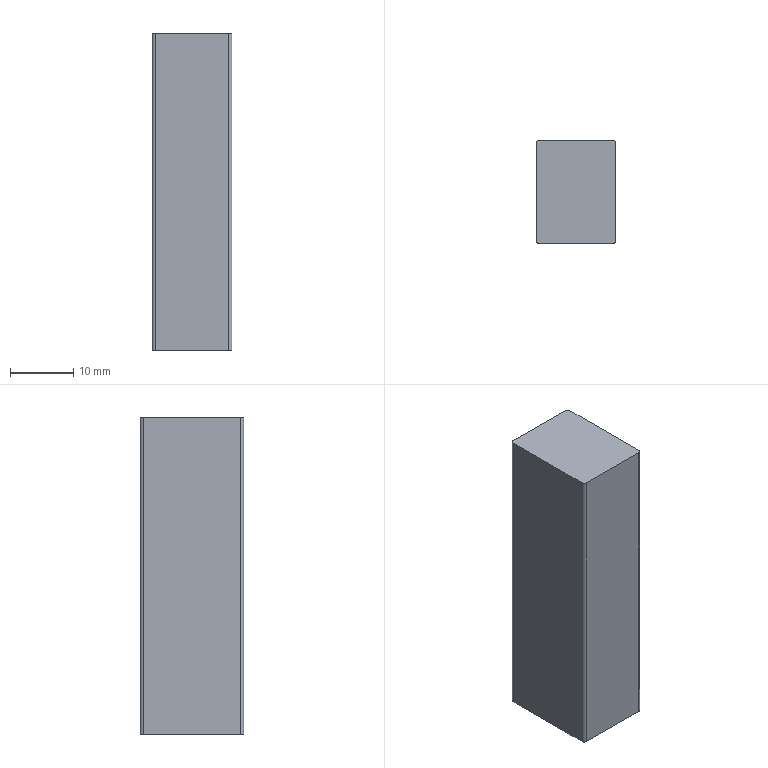Part | NX | features BREP 1 | 1 solid | 10 faces | box 12.615 x 16.326 x 50 mm | volume 10287 mm3 | plane 6 | cylinder 4 | commonest cylinder face diameters 1 x4
STEP:
#1=CARTESIAN_POINT('',(-5.808,8.163,-40.6));
#2=VERTEX_POINT('',#1);
#3=CARTESIAN_POINT('',(-6.308,7.663,-40.6));
#4=VERTEX_POINT('',#3);
#5=CARTESIAN_POINT('',(-5.808,7.663,-40.6));
#6=DIRECTION('',(0.,0.,1.));
#7=DIRECTION('',(1.,0.,0.));
#8=AXIS2_PLACEMENT_3D('',#5,#6,#7);
#9=CIRCLE('',#8,0.5);
#10=EDGE_CURVE('',#2,#4,#9,.T.);
#11=ORIENTED_EDGE('',*,*,#10,.F.);
#12=CARTESIAN_POINT('',(-5.808,8.163,-90.6));
#13=VERTEX_POINT('',#12);
#14=CARTESIAN_POINT('',(-5.808,8.163,-90.6));
#15=DIRECTION('',(0.,0.,1.));
#16=VECTOR('',#15,1000.);
#17=LINE('',#14,#16);
#18=EDGE_CURVE('',#13,#2,#17,.T.);
#19=ORIENTED_EDGE('',*,*,#18,.F.);
#20=CARTESIAN_POINT('',(-6.308,7.663,-90.6));
#21=VERTEX_POINT('',#20);
#22=CARTESIAN_POINT('',(-5.808,7.663,-90.6));
#23=DIRECTION('',(0.,0.,1.));
#24=DIRECTION('',(1.,0.,0.));
#25=AXIS2_PLACEMENT_3D('',#22,#23,#24);
#26=CIRCLE('',#25,0.5);
#27=EDGE_CURVE('',#13,#21,#26,.T.);
#28=ORIENTED_EDGE('',*,*,#27,.T.);
#29=CARTESIAN_POINT('',(-6.308,7.663,-90.6));
#30=DIRECTION('',(0.,0.,1.));
#31=VECTOR('',#30,1000.);
#32=LINE('',#29,#31);
#33=EDGE_CURVE('',#21,#4,#32,.T.);
#34=ORIENTED_EDGE('',*,*,#33,.T.);
#35=EDGE_LOOP('',(#11,#19,#28,#34));
#36=FACE_BOUND('',#35,.T.);
#37=CARTESIAN_POINT('',(-5.808,7.663,-90.6));
#38=DIRECTION('',(0.,0.,1.));
#39=DIRECTION('',(-1.,0.,0.));
#40=AXIS2_PLACEMENT_3D('',#37,#38,#39);
#41=CYLINDRICAL_SURFACE('',#40,0.5);
#42=ADVANCED_FACE('',(#36),#41,.T.);
#43=CARTESIAN_POINT('',(-6.308,-7.663,-40.6));
#44=VERTEX_POINT('',#43);
#45=CARTESIAN_POINT('',(-6.308,-7.663,-40.6));
#46=DIRECTION('',(0.,1.,0.));
#47=VECTOR('',#46,1000.);
#48=LINE('',#45,#47);
#49=EDGE_CURVE('',#44,#4,#48,.T.);
#50=ORIENTED_EDGE('',*,*,#49,.T.);
#51=ORIENTED_EDGE('',*,*,#33,.F.);
#52=CARTESIAN_POINT('',(-6.308,-7.663,-90.6));
#53=VERTEX_POINT('',#52);
#54=CARTESIAN_POINT('',(-6.308,-7.663,-90.6));
#55=DIRECTION('',(0.,1.,0.));
#56=VECTOR('',#55,1000.);
#57=LINE('',#54,#56);
#58=EDGE_CURVE('',#53,#21,#57,.T.);
#59=ORIENTED_EDGE('',*,*,#58,.F.);
#60=CARTESIAN_POINT('',(-6.308,-7.663,-90.6));
#61=DIRECTION('',(0.,0.,1.));
#62=VECTOR('',#61,1000.);
#63=LINE('',#60,#62);
#64=EDGE_CURVE('',#53,#44,#63,.T.);
#65=ORIENTED_EDGE('',*,*,#64,.T.);
#66=EDGE_LOOP('',(#50,#51,#59,#65));
#67=FACE_BOUND('',#66,.T.);
#68=CARTESIAN_POINT('',(-6.308,-7.663,-90.6));
#69=DIRECTION('',(1.,0.,0.));
#70=DIRECTION('',(0.,0.,1.));
#71=AXIS2_PLACEMENT_3D('',#68,#69,#70);
#72=PLANE('',#71);
#73=ADVANCED_FACE('',(#67),#72,.F.);
#74=CARTESIAN_POINT('',(-5.808,-8.163,-40.6));
#75=VERTEX_POINT('',#74);
#76=CARTESIAN_POINT('',(-5.808,-7.663,-40.6));
#77=DIRECTION('',(0.,0.,1.));
#78=DIRECTION('',(1.,0.,0.));
#79=AXIS2_PLACEMENT_3D('',#76,#77,#78);
#80=CIRCLE('',#79,0.5);
#81=EDGE_CURVE('',#44,#75,#80,.T.);
#82=ORIENTED_EDGE('',*,*,#81,.F.);
#83=ORIENTED_EDGE('',*,*,#64,.F.);
#84=CARTESIAN_POINT('',(-5.808,-8.163,-90.6));
#85=VERTEX_POINT('',#84);
#86=CARTESIAN_POINT('',(-5.808,-7.663,-90.6));
#87=DIRECTION('',(0.,0.,1.));
#88=DIRECTION('',(1.,0.,0.));
#89=AXIS2_PLACEMENT_3D('',#86,#87,#88);
#90=CIRCLE('',#89,0.5);
#91=EDGE_CURVE('',#53,#85,#90,.T.);
#92=ORIENTED_EDGE('',*,*,#91,.T.);
#93=CARTESIAN_POINT('',(-5.808,-8.163,-90.6));
#94=DIRECTION('',(0.,0.,1.));
#95=VECTOR('',#94,1000.);
#96=LINE('',#93,#95);
#97=EDGE_CURVE('',#85,#75,#96,.T.);
#98=ORIENTED_EDGE('',*,*,#97,.T.);
#99=EDGE_LOOP('',(#82,#83,#92,#98));
#100=FACE_BOUND('',#99,.T.);
#101=CARTESIAN_POINT('',(-5.808,-7.663,-90.6));
#102=DIRECTION('',(0.,0.,1.));
#103=DIRECTION('',(-1.,0.,0.));
#104=AXIS2_PLACEMENT_3D('',#101,#102,#103);
#105=CYLINDRICAL_SURFACE('',#104,0.5);
#106=ADVANCED_FACE('',(#100),#105,.T.);
#107=CARTESIAN_POINT('',(5.808,-8.163,-40.6));
#108=VERTEX_POINT('',#107);
#109=CARTESIAN_POINT('',(5.808,-8.163,-40.6));
#110=DIRECTION('',(-1.,0.,0.));
#111=VECTOR('',#110,1000.);
#112=LINE('',#109,#111);
#113=EDGE_CURVE('',#108,#75,#112,.T.);
#114=ORIENTED_EDGE('',*,*,#113,.T.);
#115=ORIENTED_EDGE('',*,*,#97,.F.);
#116=CARTESIAN_POINT('',(5.808,-8.163,-90.6));
#117=VERTEX_POINT('',#116);
#118=CARTESIAN_POINT('',(5.808,-8.163,-90.6));
#119=DIRECTION('',(-1.,0.,0.));
#120=VECTOR('',#119,1000.);
#121=LINE('',#118,#120);
#122=EDGE_CURVE('',#117,#85,#121,.T.);
#123=ORIENTED_EDGE('',*,*,#122,.F.);
#124=CARTESIAN_POINT('',(5.808,-8.163,-90.6));
#125=DIRECTION('',(0.,0.,1.));
#126=VECTOR('',#125,1000.);
#127=LINE('',#124,#126);
#128=EDGE_CURVE('',#117,#108,#127,.T.);
#129=ORIENTED_EDGE('',*,*,#128,.T.);
#130=EDGE_LOOP('',(#114,#115,#123,#129));
#131=FACE_BOUND('',#130,.T.);
#132=CARTESIAN_POINT('',(5.808,-8.163,-90.6));
#133=DIRECTION('',(0.,1.,0.));
#134=DIRECTION('',(0.,0.,-1.));
#135=AXIS2_PLACEMENT_3D('',#132,#133,#134);
#136=PLANE('',#135);
#137=ADVANCED_FACE('',(#131),#136,.F.);
#138=CARTESIAN_POINT('',(6.308,-7.663,-40.6));
#139=VERTEX_POINT('',#138);
#140=CARTESIAN_POINT('',(5.808,-7.663,-40.6));
#141=DIRECTION('',(0.,0.,1.));
#142=DIRECTION('',(1.,0.,0.));
#143=AXIS2_PLACEMENT_3D('',#140,#141,#142);
#144=CIRCLE('',#143,0.5);
#145=EDGE_CURVE('',#108,#139,#144,.T.);
#146=ORIENTED_EDGE('',*,*,#145,.F.);
#147=ORIENTED_EDGE('',*,*,#128,.F.);
#148=CARTESIAN_POINT('',(6.308,-7.663,-90.6));
#149=VERTEX_POINT('',#148);
#150=CARTESIAN_POINT('',(5.808,-7.663,-90.6));
#151=DIRECTION('',(0.,0.,1.));
#152=DIRECTION('',(1.,0.,0.));
#153=AXIS2_PLACEMENT_3D('',#150,#151,#152);
#154=CIRCLE('',#153,0.5);
#155=EDGE_CURVE('',#117,#149,#154,.T.);
#156=ORIENTED_EDGE('',*,*,#155,.T.);
#157=CARTESIAN_POINT('',(6.308,-7.663,-90.6));
#158=DIRECTION('',(0.,0.,1.));
#159=VECTOR('',#158,1000.);
#160=LINE('',#157,#159);
#161=EDGE_CURVE('',#149,#139,#160,.T.);
#162=ORIENTED_EDGE('',*,*,#161,.T.);
#163=EDGE_LOOP('',(#146,#147,#156,#162));
#164=FACE_BOUND('',#163,.T.);
#165=CARTESIAN_POINT('',(5.808,-7.663,-90.6));
#166=DIRECTION('',(0.,0.,1.));
#167=DIRECTION('',(-1.,0.,0.));
#168=AXIS2_PLACEMENT_3D('',#165,#166,#167);
#169=CYLINDRICAL_SURFACE('',#168,0.5);
#170=ADVANCED_FACE('',(#164),#169,.T.);
#171=CARTESIAN_POINT('',(6.308,7.663,-40.6));
#172=VERTEX_POINT('',#171);
#173=CARTESIAN_POINT('',(6.308,7.663,-40.6));
#174=DIRECTION('',(0.,-1.,0.));
#175=VECTOR('',#174,1000.);
#176=LINE('',#173,#175);
#177=EDGE_CURVE('',#172,#139,#176,.T.);
#178=ORIENTED_EDGE('',*,*,#177,.T.);
#179=ORIENTED_EDGE('',*,*,#161,.F.);
#180=CARTESIAN_POINT('',(6.308,7.663,-90.6));
#181=VERTEX_POINT('',#180);
#182=CARTESIAN_POINT('',(6.308,7.663,-90.6));
#183=DIRECTION('',(0.,-1.,0.));
#184=VECTOR('',#183,1000.);
#185=LINE('',#182,#184);
#186=EDGE_CURVE('',#181,#149,#185,.T.);
#187=ORIENTED_EDGE('',*,*,#186,.F.);
#188=CARTESIAN_POINT('',(6.308,7.663,-90.6));
#189=DIRECTION('',(0.,0.,1.));
#190=VECTOR('',#189,1000.);
#191=LINE('',#188,#190);
#192=EDGE_CURVE('',#181,#172,#191,.T.);
#193=ORIENTED_EDGE('',*,*,#192,.T.);
#194=EDGE_LOOP('',(#178,#179,#187,#193));
#195=FACE_BOUND('',#194,.T.);
#196=CARTESIAN_POINT('',(6.308,7.663,-90.6));
#197=DIRECTION('',(-1.,0.,0.));
#198=DIRECTION('',(0.,1.,0.));
#199=AXIS2_PLACEMENT_3D('',#196,#197,#198);
#200=PLANE('',#199);
#201=ADVANCED_FACE('',(#195),#200,.F.);
#202=CARTESIAN_POINT('',(5.808,8.163,-40.6));
#203=VERTEX_POINT('',#202);
#204=CARTESIAN_POINT('',(5.808,7.663,-40.6));
#205=DIRECTION('',(0.,0.,1.));
#206=DIRECTION('',(1.,0.,0.));
#207=AXIS2_PLACEMENT_3D('',#204,#205,#206);
#208=CIRCLE('',#207,0.5);
#209=EDGE_CURVE('',#172,#203,#208,.T.);
#210=ORIENTED_EDGE('',*,*,#209,.F.);
#211=ORIENTED_EDGE('',*,*,#192,.F.);
#212=CARTESIAN_POINT('',(5.808,8.163,-90.6));
#213=VERTEX_POINT('',#212);
#214=CARTESIAN_POINT('',(5.808,7.663,-90.6));
#215=DIRECTION('',(0.,0.,1.));
#216=DIRECTION('',(1.,0.,0.));
#217=AXIS2_PLACEMENT_3D('',#214,#215,#216);
#218=CIRCLE('',#217,0.5);
#219=EDGE_CURVE('',#181,#213,#218,.T.);
#220=ORIENTED_EDGE('',*,*,#219,.T.);
#221=CARTESIAN_POINT('',(5.808,8.163,-90.6));
#222=DIRECTION('',(0.,0.,1.));
#223=VECTOR('',#222,1000.);
#224=LINE('',#221,#223);
#225=EDGE_CURVE('',#213,#203,#224,.T.);
#226=ORIENTED_EDGE('',*,*,#225,.T.);
#227=EDGE_LOOP('',(#210,#211,#220,#226));
#228=FACE_BOUND('',#227,.T.);
#229=CARTESIAN_POINT('',(5.808,7.663,-90.6));
#230=DIRECTION('',(0.,0.,1.));
#231=DIRECTION('',(-1.,0.,0.));
#232=AXIS2_PLACEMENT_3D('',#229,#230,#231);
#233=CYLINDRICAL_SURFACE('',#232,0.5);
#234=ADVANCED_FACE('',(#228),#233,.T.);
#235=CARTESIAN_POINT('',(-5.808,8.163,-40.6));
#236=DIRECTION('',(1.,0.,0.));
#237=VECTOR('',#236,1000.);
#238=LINE('',#235,#237);
#239=EDGE_CURVE('',#2,#203,#238,.T.);
#240=ORIENTED_EDGE('',*,*,#239,.T.);
#241=ORIENTED_EDGE('',*,*,#225,.F.);
#242=CARTESIAN_POINT('',(-5.808,8.163,-90.6));
#243=DIRECTION('',(1.,0.,0.));
#244=VECTOR('',#243,1000.);
#245=LINE('',#242,#244);
#246=EDGE_CURVE('',#13,#213,#245,.T.);
#247=ORIENTED_EDGE('',*,*,#246,.F.);
#248=ORIENTED_EDGE('',*,*,#18,.T.);
#249=EDGE_LOOP('',(#240,#241,#247,#248));
#250=FACE_BOUND('',#249,.T.);
#251=CARTESIAN_POINT('',(-5.808,8.163,-90.6));
#252=DIRECTION('',(0.,-1.,0.));
#253=DIRECTION('',(-1.,0.,0.));
#254=AXIS2_PLACEMENT_3D('',#251,#252,#253);
#255=PLANE('',#254);
#256=ADVANCED_FACE('',(#250),#255,.F.);
#257=ORIENTED_EDGE('',*,*,#27,.F.);
#258=ORIENTED_EDGE('',*,*,#246,.T.);
#259=ORIENTED_EDGE('',*,*,#219,.F.);
#260=ORIENTED_EDGE('',*,*,#186,.T.);
#261=ORIENTED_EDGE('',*,*,#155,.F.);
#262=ORIENTED_EDGE('',*,*,#122,.T.);
#263=ORIENTED_EDGE('',*,*,#91,.F.);
#264=ORIENTED_EDGE('',*,*,#58,.T.);
#265=EDGE_LOOP('',(#257,#258,#259,#260,#261,#262,#263,#264));
#266=FACE_BOUND('',#265,.T.);
#267=CARTESIAN_POINT('',(-5.808,7.663,-90.6));
#268=DIRECTION('',(0.,0.,1.));
#269=DIRECTION('',(-1.,0.,0.));
#270=AXIS2_PLACEMENT_3D('',#267,#268,#269);
#271=PLANE('',#270);
#272=ADVANCED_FACE('',(#266),#271,.F.);
#273=ORIENTED_EDGE('',*,*,#10,.T.);
#274=ORIENTED_EDGE('',*,*,#49,.F.);
#275=ORIENTED_EDGE('',*,*,#81,.T.);
#276=ORIENTED_EDGE('',*,*,#113,.F.);
#277=ORIENTED_EDGE('',*,*,#145,.T.);
#278=ORIENTED_EDGE('',*,*,#177,.F.);
#279=ORIENTED_EDGE('',*,*,#209,.T.);
#280=ORIENTED_EDGE('',*,*,#239,.F.);
#281=EDGE_LOOP('',(#273,#274,#275,#276,#277,#278,#279,#280));
#282=FACE_BOUND('',#281,.T.);
#283=CARTESIAN_POINT('',(-5.808,7.663,-40.6));
#284=DIRECTION('',(0.,0.,1.));
#285=DIRECTION('',(-1.,0.,0.));
#286=AXIS2_PLACEMENT_3D('',#283,#284,#285);
#287=PLANE('',#286);
#288=ADVANCED_FACE('',(#282),#287,.T.);
#289=CLOSED_SHELL('',(#42,#73,#106,#137,#170,#201,#234,#256,#272,#288));
#290=MANIFOLD_SOLID_BREP('',#289);
#291=(LENGTH_UNIT()NAMED_UNIT(*)SI_UNIT(.MILLI.,.METRE.));
#292=UNCERTAINTY_MEASURE_WITH_UNIT(LENGTH_MEASURE(0.00001),#291,'','');
#293=(NAMED_UNIT(*)PLANE_ANGLE_UNIT()SI_UNIT($,.RADIAN.));
#294=(NAMED_UNIT(*)SI_UNIT($,.STERADIAN.)SOLID_ANGLE_UNIT());
#295=(GEOMETRIC_REPRESENTATION_CONTEXT(3)GLOBAL_UNCERTAINTY_ASSIGNED_CONTEXT((#292))GLOBAL_UNIT_ASSIGNED_CONTEXT((#291,#293,#294))REPRESENTATION_CONTEXT('',''));
#296=ADVANCED_BREP_SHAPE_REPRESENTATION('',(#290),#295);